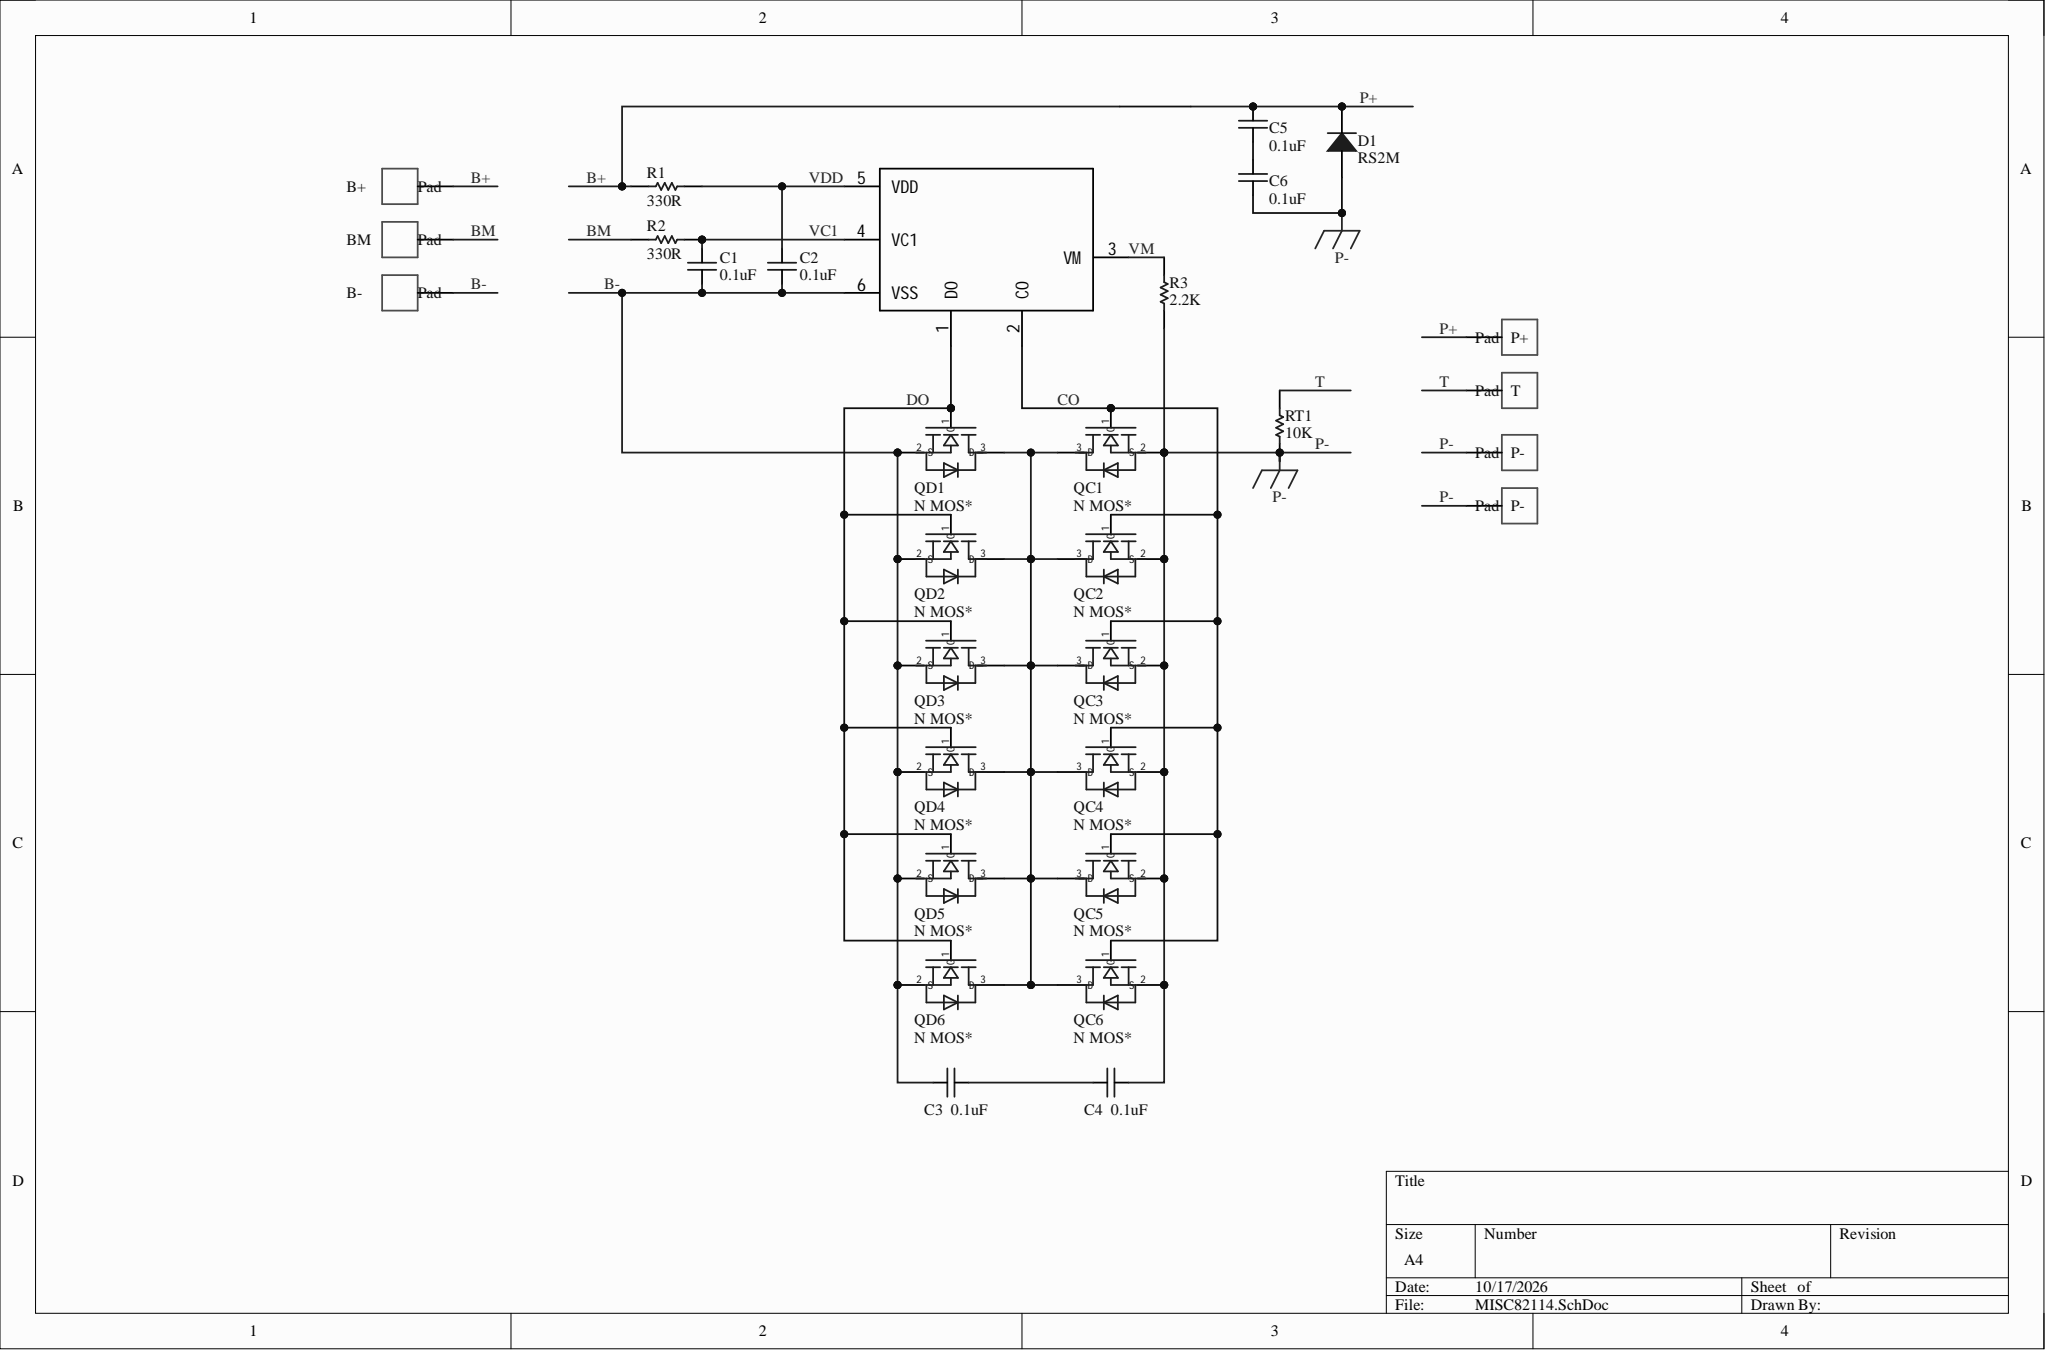Circuit board | Altium Designer | 31 parts | 13 nets
Bill of materials:
Comment,Description,Designator,Footprint,LibRef,Quantity
"Pad","Connection pad (non-through-hole)","B-, B+, BM, P-, P+, T","Pad10X8mm","Pad","7"
"0.1uF","SMD capacitor","C1, C2, C3, C4, C5, C6","C0603A","CAP","6"
"RS2M","SMD diode","D1","SMA(DO-214AC)","RS2M","1"
"N MOS*","SMD MOSFET","QC1, QC2, QC3, QC4, QC5, QC6, QD1, QD2, QD3, QD4, QD5, QD6","DFN-3x3L8(T3P)","N MOS*","12"
"330R","SMD resistor","R1, R2","R0603A","RES","2"
"2.2K","SMD resistor","R3","R0603A","RES","1"
"10K","SMD resistor","RT1","R0603A","RES","1"
"CW1025*","1-2S battery protection IC","U1","SOT23-6A","CW1025*","1"
Netlist (Protel format):
[
B+
Pad10X8mm
Pad



]
[
B-
Pad10X8mm
Pad



]
[
BM
Pad10X8mm
Pad



]
[
C1
C0603A
0.1uF



]
[
C2
C0603A
0.1uF



]
[
C3
C0603A
0.1uF



]
[
C4
C0603A
0.1uF



]
[
C5
C0603A
0.1uF



]
[
C6
C0603A
0.1uF



]
[
D1
SMA(DO-214AC)
RS2M



]
[
P+
Pad10X8mm
Pad



]
[
P-
Pad10X8mm
Pad



]
[
P-
Pad10X8mm
Pad



]
[
QC1
DFN-3x3L8(T3P)
N MOS*



]
[
QC2
DFN-3x3L8(T3P)
N MOS*



]
[
QC3
DFN-3x3L8(T3P)
N MOS*



]
[
QC4
DFN-3x3L8(T3P)
N MOS*



]
[
QC5
DFN-3x3L8(T3P)
N MOS*



]
[
QC6
DFN-3x3L8(T3P)
N MOS*



]
[
QD1
DFN-3x3L8(T3P)
N MOS*



]
[
QD2
DFN-3x3L8(T3P)
N MOS*



]
[
QD3
DFN-3x3L8(T3P)
N MOS*



]
[
QD4
DFN-3x3L8(T3P)
N MOS*



]
[
QD5
DFN-3x3L8(T3P)
N MOS*



]
[
QD6
DFN-3x3L8(T3P)
N MOS*



]
[
R1
R0603A
330R



]
[
R2
R0603A
330R



]
[
R3
R0603A
2.2K



]
[
RT1
R0603A
10K



]
[
T
Pad10X8mm
Pad



]
[
U1
SOT23-6A
CW1025*



]
(
VM
R3-2
U1-3
)
(
VDD
C2-2
R1-2
U1-5
)
(
VC1
C1-2
R2-2
U1-4
)
(
T
RT1-2
T-1
)
(
P-
C4-1
C6-2
D1-2
P--1
P--1
QC1-2
QC2-2
QC3-2
QC4-2
QC5-2
QC6-2
R3-1
RT1-1
)
(
NetQC1_3
QC1-3
QC2-3
QC3-3
QC4-3
QC5-3
QC6-3
QD1-3
QD2-3
QD3-3
QD4-3
QD5-3
QD6-3
)
(
NetC5_2
C5-2
C6-1
)
(
NetC3_1
C3-1
C4-2
)
(
DO
QD1-1
QD2-1
QD3-1
QD4-1
QD5-1
QD6-1
U1-1
)
(
CO
QC1-1
QC2-1
QC3-1
QC4-1
QC5-1
QC6-1
U1-2
)
(
BM
BM-1
R2-1
)
(
B-
B--1
C1-1
C2-1
C3-2
QD1-2
QD2-2
QD3-2
QD4-2
QD5-2
QD6-2
U1-6
)
(
B+
B+-1
C5-1
D1-1
P+-1
R1-1
)